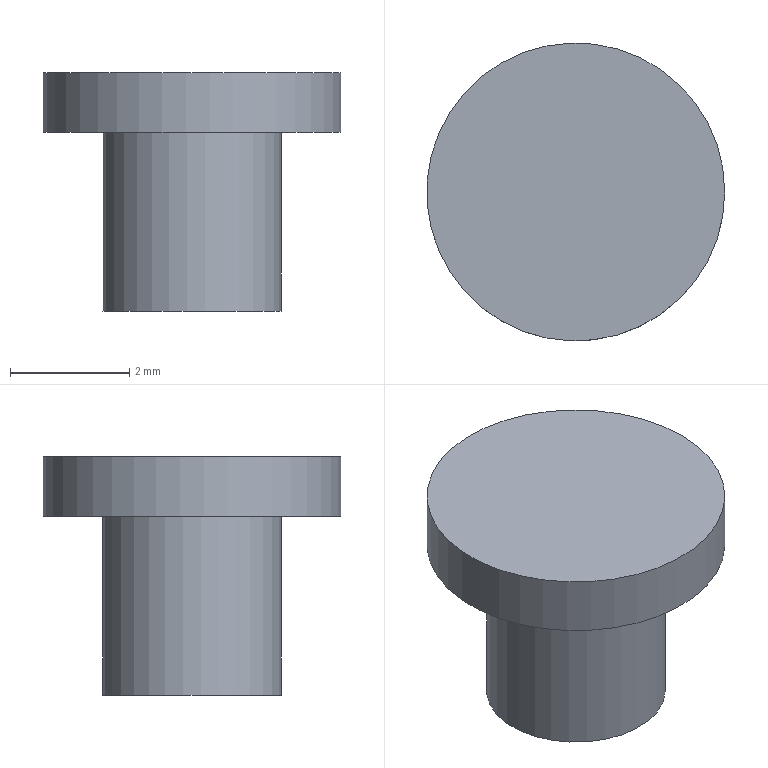Part | NX | features CYLINDER 2, DATUM_CSYS 1, UNITE 1 | 1 solid | 5 faces | box 5 x 5 x 4 mm | volume 40.841 mm3 | plane 3 | cylinder 2 | commonest cylinder face diameters 3 x1 5 x1
STEP:
#1=CARTESIAN_POINT('',(1.5,0.,0.));
#2=VERTEX_POINT('',#1);
#3=CARTESIAN_POINT('',(0.,0.,0.));
#4=DIRECTION('',(0.,0.,1.));
#5=DIRECTION('',(1.,0.,0.));
#6=AXIS2_PLACEMENT_3D('',#3,#4,#5);
#7=CIRCLE('',#6,1.5);
#8=EDGE_CURVE('',#2,#2,#7,.T.);
#9=ORIENTED_EDGE('',*,*,#8,.F.);
#10=EDGE_LOOP('',(#9));
#11=FACE_BOUND('',#10,.T.);
#12=CARTESIAN_POINT('',(0.,0.,0.));
#13=DIRECTION('',(0.,0.,-1.));
#14=DIRECTION('',(-1.,0.,0.));
#15=AXIS2_PLACEMENT_3D('',#12,#13,#14);
#16=PLANE('',#15);
#17=ADVANCED_FACE('',(#11),#16,.T.);
#18=CARTESIAN_POINT('',(1.5,0.,3.));
#19=VERTEX_POINT('',#18);
#20=CARTESIAN_POINT('',(0.,0.,3.));
#21=DIRECTION('',(0.,0.,-1.));
#22=DIRECTION('',(1.,0.,0.));
#23=AXIS2_PLACEMENT_3D('',#20,#21,#22);
#24=CIRCLE('',#23,1.5);
#25=EDGE_CURVE('',#19,#19,#24,.T.);
#26=ORIENTED_EDGE('',*,*,#25,.T.);
#27=EDGE_LOOP('',(#26));
#28=FACE_BOUND('',#27,.T.);
#29=ORIENTED_EDGE('',*,*,#8,.T.);
#30=EDGE_LOOP('',(#29));
#31=FACE_BOUND('',#30,.T.);
#32=CARTESIAN_POINT('',(0.,0.,0.));
#33=DIRECTION('',(0.,0.,1.));
#34=DIRECTION('',(1.,0.,0.));
#35=AXIS2_PLACEMENT_3D('',#32,#33,#34);
#36=CYLINDRICAL_SURFACE('',#35,1.5);
#37=ADVANCED_FACE('',(#28,#31),#36,.T.);
#38=CARTESIAN_POINT('',(2.5,0.,4.));
#39=VERTEX_POINT('',#38);
#40=CARTESIAN_POINT('',(0.,0.,4.));
#41=DIRECTION('',(0.,0.,-1.));
#42=DIRECTION('',(1.,0.,0.));
#43=AXIS2_PLACEMENT_3D('',#40,#41,#42);
#44=CIRCLE('',#43,2.5);
#45=EDGE_CURVE('',#39,#39,#44,.T.);
#46=ORIENTED_EDGE('',*,*,#45,.F.);
#47=EDGE_LOOP('',(#46));
#48=FACE_BOUND('',#47,.T.);
#49=CARTESIAN_POINT('',(0.,0.,4.));
#50=DIRECTION('',(0.,0.,1.));
#51=DIRECTION('',(1.,0.,0.));
#52=AXIS2_PLACEMENT_3D('',#49,#50,#51);
#53=PLANE('',#52);
#54=ADVANCED_FACE('',(#48),#53,.T.);
#55=ORIENTED_EDGE('',*,*,#25,.F.);
#56=EDGE_LOOP('',(#55));
#57=FACE_BOUND('',#56,.T.);
#58=CARTESIAN_POINT('',(2.5,0.,3.));
#59=VERTEX_POINT('',#58);
#60=CARTESIAN_POINT('',(0.,0.,3.));
#61=DIRECTION('',(0.,0.,1.));
#62=DIRECTION('',(1.,0.,0.));
#63=AXIS2_PLACEMENT_3D('',#60,#61,#62);
#64=CIRCLE('',#63,2.5);
#65=EDGE_CURVE('',#59,#59,#64,.T.);
#66=ORIENTED_EDGE('',*,*,#65,.F.);
#67=EDGE_LOOP('',(#66));
#68=FACE_BOUND('',#67,.T.);
#69=CARTESIAN_POINT('',(0.,0.,3.));
#70=DIRECTION('',(0.,0.,-1.));
#71=DIRECTION('',(-1.,0.,0.));
#72=AXIS2_PLACEMENT_3D('',#69,#70,#71);
#73=PLANE('',#72);
#74=ADVANCED_FACE('',(#57,#68),#73,.T.);
#75=ORIENTED_EDGE('',*,*,#45,.T.);
#76=EDGE_LOOP('',(#75));
#77=FACE_BOUND('',#76,.T.);
#78=ORIENTED_EDGE('',*,*,#65,.T.);
#79=EDGE_LOOP('',(#78));
#80=FACE_BOUND('',#79,.T.);
#81=CARTESIAN_POINT('',(0.,0.,3.));
#82=DIRECTION('',(0.,0.,1.));
#83=DIRECTION('',(1.,0.,0.));
#84=AXIS2_PLACEMENT_3D('',#81,#82,#83);
#85=CYLINDRICAL_SURFACE('',#84,2.5);
#86=ADVANCED_FACE('',(#77,#80),#85,.T.);
#87=CLOSED_SHELL('',(#17,#37,#54,#74,#86));
#88=MANIFOLD_SOLID_BREP('',#87);
#89=(LENGTH_UNIT()NAMED_UNIT(*)SI_UNIT(.MILLI.,.METRE.));
#90=UNCERTAINTY_MEASURE_WITH_UNIT(LENGTH_MEASURE(0.00001),#89,'','');
#91=(NAMED_UNIT(*)PLANE_ANGLE_UNIT()SI_UNIT($,.RADIAN.));
#92=(NAMED_UNIT(*)SI_UNIT($,.STERADIAN.)SOLID_ANGLE_UNIT());
#93=(GEOMETRIC_REPRESENTATION_CONTEXT(3)GLOBAL_UNCERTAINTY_ASSIGNED_CONTEXT((#90))GLOBAL_UNIT_ASSIGNED_CONTEXT((#89,#91,#92))REPRESENTATION_CONTEXT('',''));
#94=ADVANCED_BREP_SHAPE_REPRESENTATION('',(#88),#93);